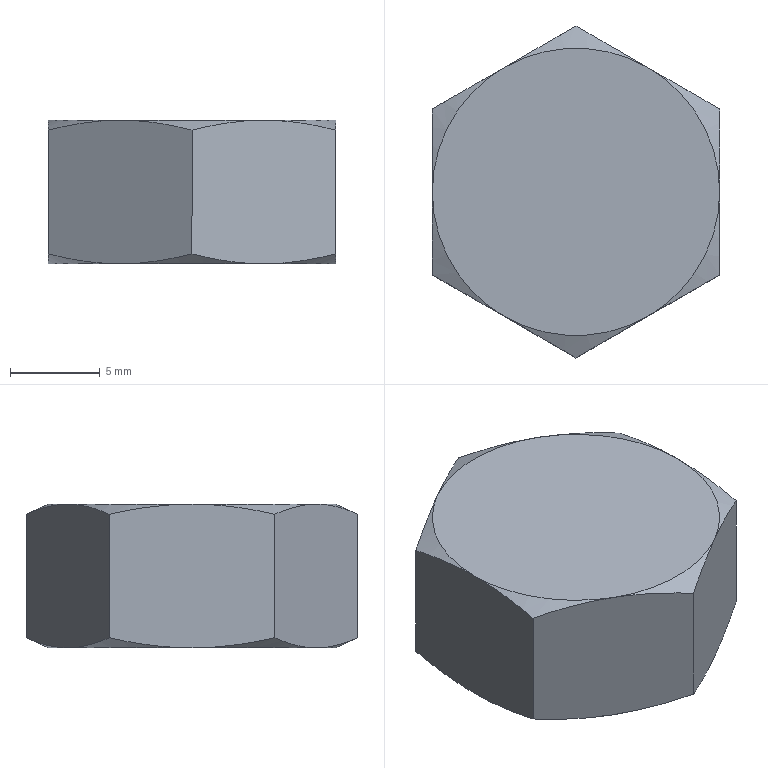Part | NX | features BREP 1 | 1 solid | 20 faces | box 16 x 18.475 x 8 mm | volume 1767 mm3 | cone 12 | plane 8
STEP:
#1=CARTESIAN_POINT('',(0.,-9.238,39.56));
#2=VERTEX_POINT('',#1);
#3=CARTESIAN_POINT('',(-4.,-6.928,39.));
#4=VERTEX_POINT('',#3);
#5=CARTESIAN_POINT('',(0.,-9.238,39.56));
#6=CARTESIAN_POINT('',(-1.317,-8.477,39.216));
#7=CARTESIAN_POINT('',(-2.647,-7.709,39.));
#8=CARTESIAN_POINT('',(-4.,-6.928,39.));
#9=B_SPLINE_CURVE_WITH_KNOTS('',3,(#5,#6,#7,#8),.UNSPECIFIED.,.F.,.F.,(4,4),(0.,0.004653),.UNSPECIFIED.);
#10=EDGE_CURVE('',#2,#4,#9,.T.);
#11=ORIENTED_EDGE('',*,*,#10,.T.);
#12=CARTESIAN_POINT('',(4.,-6.928,39.));
#13=VERTEX_POINT('',#12);
#14=CARTESIAN_POINT('',(0.,0.,39.));
#15=DIRECTION('',(0.,0.,-1.));
#16=DIRECTION('',(0.5,-0.866,0.));
#17=AXIS2_PLACEMENT_3D('',#14,#15,#16);
#18=CIRCLE('',#17,8.);
#19=EDGE_CURVE('',#13,#4,#18,.T.);
#20=ORIENTED_EDGE('',*,*,#19,.F.);
#21=CARTESIAN_POINT('',(4.,-6.928,39.));
#22=CARTESIAN_POINT('',(2.647,-7.709,39.));
#23=CARTESIAN_POINT('',(1.317,-8.477,39.216));
#24=CARTESIAN_POINT('',(0.,-9.238,39.56));
#25=B_SPLINE_CURVE_WITH_KNOTS('',3,(#21,#22,#23,#24),.UNSPECIFIED.,.F.,.F.,(4,4),(0.,0.004653),.UNSPECIFIED.);
#26=EDGE_CURVE('',#13,#2,#25,.T.);
#27=ORIENTED_EDGE('',*,*,#26,.T.);
#28=EDGE_LOOP('',(#11,#20,#27));
#29=FACE_BOUND('',#28,.T.);
#30=CARTESIAN_POINT('',(0.,0.,39.28));
#31=DIRECTION('',(0.,0.,1.));
#32=DIRECTION('',(-1.,0.,0.));
#33=AXIS2_PLACEMENT_3D('',#30,#31,#32);
#34=CONICAL_SURFACE('',#33,8.619,1.146);
#35=ADVANCED_FACE('',(#29),#34,.T.);
#36=CARTESIAN_POINT('',(0.,-9.238,46.44));
#37=VERTEX_POINT('',#36);
#38=CARTESIAN_POINT('',(0.,-9.238,39.56));
#39=DIRECTION('',(0.,0.,1.));
#40=VECTOR('',#39,1000.);
#41=LINE('',#38,#40);
#42=EDGE_CURVE('',#2,#37,#41,.T.);
#43=ORIENTED_EDGE('',*,*,#42,.F.);
#44=ORIENTED_EDGE('',*,*,#26,.F.);
#45=CARTESIAN_POINT('',(8.,-4.619,39.56));
#46=VERTEX_POINT('',#45);
#47=CARTESIAN_POINT('',(8.,-4.619,39.56));
#48=CARTESIAN_POINT('',(6.683,-5.379,39.216));
#49=CARTESIAN_POINT('',(5.353,-6.147,39.));
#50=CARTESIAN_POINT('',(4.,-6.928,39.));
#51=B_SPLINE_CURVE_WITH_KNOTS('',3,(#47,#48,#49,#50),.UNSPECIFIED.,.F.,.F.,(4,4),(0.,0.004653),.UNSPECIFIED.);
#52=EDGE_CURVE('',#46,#13,#51,.T.);
#53=ORIENTED_EDGE('',*,*,#52,.F.);
#54=CARTESIAN_POINT('',(8.,-4.619,46.44));
#55=VERTEX_POINT('',#54);
#56=CARTESIAN_POINT('',(8.,-4.619,39.56));
#57=DIRECTION('',(0.,0.,1.));
#58=VECTOR('',#57,1000.);
#59=LINE('',#56,#58);
#60=EDGE_CURVE('',#46,#55,#59,.T.);
#61=ORIENTED_EDGE('',*,*,#60,.T.);
#62=CARTESIAN_POINT('',(4.,-6.928,47.));
#63=VERTEX_POINT('',#62);
#64=CARTESIAN_POINT('',(4.,-6.928,47.));
#65=CARTESIAN_POINT('',(5.353,-6.147,47.));
#66=CARTESIAN_POINT('',(6.683,-5.379,46.784));
#67=CARTESIAN_POINT('',(8.,-4.619,46.44));
#68=B_SPLINE_CURVE_WITH_KNOTS('',3,(#64,#65,#66,#67),.UNSPECIFIED.,.F.,.F.,(4,4),(0.,0.004653),.UNSPECIFIED.);
#69=EDGE_CURVE('',#63,#55,#68,.T.);
#70=ORIENTED_EDGE('',*,*,#69,.F.);
#71=CARTESIAN_POINT('',(0.,-9.238,46.44));
#72=CARTESIAN_POINT('',(1.317,-8.477,46.784));
#73=CARTESIAN_POINT('',(2.647,-7.709,47.));
#74=CARTESIAN_POINT('',(4.,-6.928,47.));
#75=B_SPLINE_CURVE_WITH_KNOTS('',3,(#71,#72,#73,#74),.UNSPECIFIED.,.F.,.F.,(4,4),(0.,0.004653),.UNSPECIFIED.);
#76=EDGE_CURVE('',#37,#63,#75,.T.);
#77=ORIENTED_EDGE('',*,*,#76,.F.);
#78=EDGE_LOOP('',(#43,#44,#53,#61,#70,#77));
#79=FACE_BOUND('',#78,.T.);
#80=CARTESIAN_POINT('',(0.,-9.238,47.));
#81=DIRECTION('',(-0.5,0.866,0.));
#82=DIRECTION('',(0.866,0.5,0.));
#83=AXIS2_PLACEMENT_3D('',#80,#81,#82);
#84=PLANE('',#83);
#85=ADVANCED_FACE('',(#79),#84,.F.);
#86=ORIENTED_EDGE('',*,*,#76,.T.);
#87=CARTESIAN_POINT('',(-4.,-6.928,47.));
#88=VERTEX_POINT('',#87);
#89=CARTESIAN_POINT('',(0.,0.,47.));
#90=DIRECTION('',(0.,0.,1.));
#91=DIRECTION('',(-0.5,-0.866,0.));
#92=AXIS2_PLACEMENT_3D('',#89,#90,#91);
#93=CIRCLE('',#92,8.);
#94=EDGE_CURVE('',#88,#63,#93,.T.);
#95=ORIENTED_EDGE('',*,*,#94,.F.);
#96=CARTESIAN_POINT('',(-4.,-6.928,47.));
#97=CARTESIAN_POINT('',(-2.647,-7.709,47.));
#98=CARTESIAN_POINT('',(-1.317,-8.477,46.784));
#99=CARTESIAN_POINT('',(0.,-9.238,46.44));
#100=B_SPLINE_CURVE_WITH_KNOTS('',3,(#96,#97,#98,#99),.UNSPECIFIED.,.F.,.F.,(4,4),(0.,0.004653),.UNSPECIFIED.);
#101=EDGE_CURVE('',#88,#37,#100,.T.);
#102=ORIENTED_EDGE('',*,*,#101,.T.);
#103=EDGE_LOOP('',(#86,#95,#102));
#104=FACE_BOUND('',#103,.T.);
#105=CARTESIAN_POINT('',(0.,0.,46.72));
#106=DIRECTION('',(0.,0.,-1.));
#107=DIRECTION('',(1.,0.,0.));
#108=AXIS2_PLACEMENT_3D('',#105,#106,#107);
#109=CONICAL_SURFACE('',#108,8.619,1.146);
#110=ADVANCED_FACE('',(#104),#109,.T.);
#111=CARTESIAN_POINT('',(-8.,-4.619,39.56));
#112=VERTEX_POINT('',#111);
#113=CARTESIAN_POINT('',(-8.,-4.619,46.44));
#114=VERTEX_POINT('',#113);
#115=CARTESIAN_POINT('',(-8.,-4.619,39.56));
#116=DIRECTION('',(0.,0.,1.));
#117=VECTOR('',#116,1000.);
#118=LINE('',#115,#117);
#119=EDGE_CURVE('',#112,#114,#118,.T.);
#120=ORIENTED_EDGE('',*,*,#119,.F.);
#121=CARTESIAN_POINT('',(-4.,-6.928,39.));
#122=CARTESIAN_POINT('',(-5.353,-6.147,39.));
#123=CARTESIAN_POINT('',(-6.683,-5.379,39.216));
#124=CARTESIAN_POINT('',(-8.,-4.619,39.56));
#125=B_SPLINE_CURVE_WITH_KNOTS('',3,(#121,#122,#123,#124),.UNSPECIFIED.,.F.,.F.,(4,4),(0.,0.004653),.UNSPECIFIED.);
#126=EDGE_CURVE('',#4,#112,#125,.T.);
#127=ORIENTED_EDGE('',*,*,#126,.F.);
#128=ORIENTED_EDGE('',*,*,#10,.F.);
#129=ORIENTED_EDGE('',*,*,#42,.T.);
#130=ORIENTED_EDGE('',*,*,#101,.F.);
#131=CARTESIAN_POINT('',(-8.,-4.619,46.44));
#132=CARTESIAN_POINT('',(-6.683,-5.379,46.784));
#133=CARTESIAN_POINT('',(-5.353,-6.147,47.));
#134=CARTESIAN_POINT('',(-4.,-6.928,47.));
#135=B_SPLINE_CURVE_WITH_KNOTS('',3,(#131,#132,#133,#134),.UNSPECIFIED.,.F.,.F.,(4,4),(0.,0.004653),.UNSPECIFIED.);
#136=EDGE_CURVE('',#114,#88,#135,.T.);
#137=ORIENTED_EDGE('',*,*,#136,.F.);
#138=EDGE_LOOP('',(#120,#127,#128,#129,#130,#137));
#139=FACE_BOUND('',#138,.T.);
#140=CARTESIAN_POINT('',(-8.,-4.619,47.));
#141=DIRECTION('',(0.5,0.866,0.));
#142=DIRECTION('',(0.866,-0.5,0.));
#143=AXIS2_PLACEMENT_3D('',#140,#141,#142);
#144=PLANE('',#143);
#145=ADVANCED_FACE('',(#139),#144,.F.);
#146=CARTESIAN_POINT('',(-8.,0.,47.));
#147=VERTEX_POINT('',#146);
#148=CARTESIAN_POINT('',(0.,0.,47.));
#149=DIRECTION('',(0.,0.,1.));
#150=DIRECTION('',(-1.,0.,0.));
#151=AXIS2_PLACEMENT_3D('',#148,#149,#150);
#152=CIRCLE('',#151,8.);
#153=EDGE_CURVE('',#147,#88,#152,.T.);
#154=ORIENTED_EDGE('',*,*,#153,.F.);
#155=CARTESIAN_POINT('',(-8.,0.,47.));
#156=CARTESIAN_POINT('',(-8.,-1.562,47.));
#157=CARTESIAN_POINT('',(-8.,-3.098,46.784));
#158=CARTESIAN_POINT('',(-8.,-4.619,46.44));
#159=B_SPLINE_CURVE_WITH_KNOTS('',3,(#155,#156,#157,#158),.UNSPECIFIED.,.F.,.F.,(4,4),(0.,0.004653),.UNSPECIFIED.);
#160=EDGE_CURVE('',#147,#114,#159,.T.);
#161=ORIENTED_EDGE('',*,*,#160,.T.);
#162=ORIENTED_EDGE('',*,*,#136,.T.);
#163=EDGE_LOOP('',(#154,#161,#162));
#164=FACE_BOUND('',#163,.T.);
#165=CARTESIAN_POINT('',(0.,0.,46.72));
#166=DIRECTION('',(0.,0.,-1.));
#167=DIRECTION('',(1.,0.,0.));
#168=AXIS2_PLACEMENT_3D('',#165,#166,#167);
#169=CONICAL_SURFACE('',#168,8.619,1.146);
#170=ADVANCED_FACE('',(#164),#169,.T.);
#171=CARTESIAN_POINT('',(-8.,4.619,39.56));
#172=VERTEX_POINT('',#171);
#173=CARTESIAN_POINT('',(-8.,4.619,46.44));
#174=VERTEX_POINT('',#173);
#175=CARTESIAN_POINT('',(-8.,4.619,39.56));
#176=DIRECTION('',(0.,0.,1.));
#177=VECTOR('',#176,1000.);
#178=LINE('',#175,#177);
#179=EDGE_CURVE('',#172,#174,#178,.T.);
#180=ORIENTED_EDGE('',*,*,#179,.F.);
#181=CARTESIAN_POINT('',(-8.,0.,39.));
#182=VERTEX_POINT('',#181);
#183=CARTESIAN_POINT('',(-8.,0.,39.));
#184=CARTESIAN_POINT('',(-8.,1.562,39.));
#185=CARTESIAN_POINT('',(-8.,3.098,39.216));
#186=CARTESIAN_POINT('',(-8.,4.619,39.56));
#187=B_SPLINE_CURVE_WITH_KNOTS('',3,(#183,#184,#185,#186),.UNSPECIFIED.,.F.,.F.,(4,4),(0.,0.004653),.UNSPECIFIED.);
#188=EDGE_CURVE('',#182,#172,#187,.T.);
#189=ORIENTED_EDGE('',*,*,#188,.F.);
#190=CARTESIAN_POINT('',(-8.,-4.619,39.56));
#191=CARTESIAN_POINT('',(-8.,-3.098,39.216));
#192=CARTESIAN_POINT('',(-8.,-1.562,39.));
#193=CARTESIAN_POINT('',(-8.,0.,39.));
#194=B_SPLINE_CURVE_WITH_KNOTS('',3,(#190,#191,#192,#193),.UNSPECIFIED.,.F.,.F.,(4,4),(0.,0.004653),.UNSPECIFIED.);
#195=EDGE_CURVE('',#112,#182,#194,.T.);
#196=ORIENTED_EDGE('',*,*,#195,.F.);
#197=ORIENTED_EDGE('',*,*,#119,.T.);
#198=ORIENTED_EDGE('',*,*,#160,.F.);
#199=CARTESIAN_POINT('',(-8.,4.619,46.44));
#200=CARTESIAN_POINT('',(-8.,3.098,46.784));
#201=CARTESIAN_POINT('',(-8.,1.562,47.));
#202=CARTESIAN_POINT('',(-8.,0.,47.));
#203=B_SPLINE_CURVE_WITH_KNOTS('',3,(#199,#200,#201,#202),.UNSPECIFIED.,.F.,.F.,(4,4),(0.,0.004653),.UNSPECIFIED.);
#204=EDGE_CURVE('',#174,#147,#203,.T.);
#205=ORIENTED_EDGE('',*,*,#204,.F.);
#206=EDGE_LOOP('',(#180,#189,#196,#197,#198,#205));
#207=FACE_BOUND('',#206,.T.);
#208=CARTESIAN_POINT('',(-8.,4.619,47.));
#209=DIRECTION('',(1.,0.,0.));
#210=DIRECTION('',(0.,-1.,0.));
#211=AXIS2_PLACEMENT_3D('',#208,#209,#210);
#212=PLANE('',#211);
#213=ADVANCED_FACE('',(#207),#212,.F.);
#214=ORIENTED_EDGE('',*,*,#204,.T.);
#215=CARTESIAN_POINT('',(-4.,6.928,47.));
#216=VERTEX_POINT('',#215);
#217=CARTESIAN_POINT('',(0.,0.,47.));
#218=DIRECTION('',(0.,0.,1.));
#219=DIRECTION('',(-0.5,0.866,0.));
#220=AXIS2_PLACEMENT_3D('',#217,#218,#219);
#221=CIRCLE('',#220,8.);
#222=EDGE_CURVE('',#216,#147,#221,.T.);
#223=ORIENTED_EDGE('',*,*,#222,.F.);
#224=CARTESIAN_POINT('',(-4.,6.928,47.));
#225=CARTESIAN_POINT('',(-5.353,6.147,47.));
#226=CARTESIAN_POINT('',(-6.683,5.379,46.784));
#227=CARTESIAN_POINT('',(-8.,4.619,46.44));
#228=B_SPLINE_CURVE_WITH_KNOTS('',3,(#224,#225,#226,#227),.UNSPECIFIED.,.F.,.F.,(4,4),(0.,0.004653),.UNSPECIFIED.);
#229=EDGE_CURVE('',#216,#174,#228,.T.);
#230=ORIENTED_EDGE('',*,*,#229,.T.);
#231=EDGE_LOOP('',(#214,#223,#230));
#232=FACE_BOUND('',#231,.T.);
#233=CARTESIAN_POINT('',(0.,0.,46.72));
#234=DIRECTION('',(0.,0.,-1.));
#235=DIRECTION('',(1.,0.,0.));
#236=AXIS2_PLACEMENT_3D('',#233,#234,#235);
#237=CONICAL_SURFACE('',#236,8.619,1.146);
#238=ADVANCED_FACE('',(#232),#237,.T.);
#239=CARTESIAN_POINT('',(0.,9.238,39.56));
#240=VERTEX_POINT('',#239);
#241=CARTESIAN_POINT('',(0.,9.238,46.44));
#242=VERTEX_POINT('',#241);
#243=CARTESIAN_POINT('',(0.,9.238,39.56));
#244=DIRECTION('',(0.,0.,1.));
#245=VECTOR('',#244,1000.);
#246=LINE('',#243,#245);
#247=EDGE_CURVE('',#240,#242,#246,.T.);
#248=ORIENTED_EDGE('',*,*,#247,.F.);
#249=CARTESIAN_POINT('',(-4.,6.928,39.));
#250=VERTEX_POINT('',#249);
#251=CARTESIAN_POINT('',(-4.,6.928,39.));
#252=CARTESIAN_POINT('',(-2.647,7.709,39.));
#253=CARTESIAN_POINT('',(-1.317,8.477,39.216));
#254=CARTESIAN_POINT('',(0.,9.238,39.56));
#255=B_SPLINE_CURVE_WITH_KNOTS('',3,(#251,#252,#253,#254),.UNSPECIFIED.,.F.,.F.,(4,4),(0.,0.004653),.UNSPECIFIED.);
#256=EDGE_CURVE('',#250,#240,#255,.T.);
#257=ORIENTED_EDGE('',*,*,#256,.F.);
#258=CARTESIAN_POINT('',(-8.,4.619,39.56));
#259=CARTESIAN_POINT('',(-6.683,5.379,39.216));
#260=CARTESIAN_POINT('',(-5.353,6.147,39.));
#261=CARTESIAN_POINT('',(-4.,6.928,39.));
#262=B_SPLINE_CURVE_WITH_KNOTS('',3,(#258,#259,#260,#261),.UNSPECIFIED.,.F.,.F.,(4,4),(0.,0.004653),.UNSPECIFIED.);
#263=EDGE_CURVE('',#172,#250,#262,.T.);
#264=ORIENTED_EDGE('',*,*,#263,.F.);
#265=ORIENTED_EDGE('',*,*,#179,.T.);
#266=ORIENTED_EDGE('',*,*,#229,.F.);
#267=CARTESIAN_POINT('',(0.,9.238,46.44));
#268=CARTESIAN_POINT('',(-1.317,8.477,46.784));
#269=CARTESIAN_POINT('',(-2.647,7.709,47.));
#270=CARTESIAN_POINT('',(-4.,6.928,47.));
#271=B_SPLINE_CURVE_WITH_KNOTS('',3,(#267,#268,#269,#270),.UNSPECIFIED.,.F.,.F.,(4,4),(0.,0.004653),.UNSPECIFIED.);
#272=EDGE_CURVE('',#242,#216,#271,.T.);
#273=ORIENTED_EDGE('',*,*,#272,.F.);
#274=EDGE_LOOP('',(#248,#257,#264,#265,#266,#273));
#275=FACE_BOUND('',#274,.T.);
#276=CARTESIAN_POINT('',(0.,9.238,47.));
#277=DIRECTION('',(0.5,-0.866,0.));
#278=DIRECTION('',(-0.866,-0.5,0.));
#279=AXIS2_PLACEMENT_3D('',#276,#277,#278);
#280=PLANE('',#279);
#281=ADVANCED_FACE('',(#275),#280,.F.);
#282=ORIENTED_EDGE('',*,*,#272,.T.);
#283=CARTESIAN_POINT('',(4.,6.928,47.));
#284=VERTEX_POINT('',#283);
#285=CARTESIAN_POINT('',(0.,0.,47.));
#286=DIRECTION('',(0.,0.,1.));
#287=DIRECTION('',(0.5,0.866,0.));
#288=AXIS2_PLACEMENT_3D('',#285,#286,#287);
#289=CIRCLE('',#288,8.);
#290=EDGE_CURVE('',#284,#216,#289,.T.);
#291=ORIENTED_EDGE('',*,*,#290,.F.);
#292=CARTESIAN_POINT('',(4.,6.928,47.));
#293=CARTESIAN_POINT('',(2.647,7.709,47.));
#294=CARTESIAN_POINT('',(1.317,8.477,46.784));
#295=CARTESIAN_POINT('',(0.,9.238,46.44));
#296=B_SPLINE_CURVE_WITH_KNOTS('',3,(#292,#293,#294,#295),.UNSPECIFIED.,.F.,.F.,(4,4),(0.,0.004653),.UNSPECIFIED.);
#297=EDGE_CURVE('',#284,#242,#296,.T.);
#298=ORIENTED_EDGE('',*,*,#297,.T.);
#299=EDGE_LOOP('',(#282,#291,#298));
#300=FACE_BOUND('',#299,.T.);
#301=CARTESIAN_POINT('',(0.,0.,46.72));
#302=DIRECTION('',(0.,0.,-1.));
#303=DIRECTION('',(1.,0.,0.));
#304=AXIS2_PLACEMENT_3D('',#301,#302,#303);
#305=CONICAL_SURFACE('',#304,8.619,1.146);
#306=ADVANCED_FACE('',(#300),#305,.T.);
#307=CARTESIAN_POINT('',(8.,4.619,39.56));
#308=VERTEX_POINT('',#307);
#309=CARTESIAN_POINT('',(8.,4.619,46.44));
#310=VERTEX_POINT('',#309);
#311=CARTESIAN_POINT('',(8.,4.619,39.56));
#312=DIRECTION('',(0.,0.,1.));
#313=VECTOR('',#312,1000.);
#314=LINE('',#311,#313);
#315=EDGE_CURVE('',#308,#310,#314,.T.);
#316=ORIENTED_EDGE('',*,*,#315,.F.);
#317=CARTESIAN_POINT('',(4.,6.928,39.));
#318=VERTEX_POINT('',#317);
#319=CARTESIAN_POINT('',(4.,6.928,39.));
#320=CARTESIAN_POINT('',(5.353,6.147,39.));
#321=CARTESIAN_POINT('',(6.683,5.379,39.216));
#322=CARTESIAN_POINT('',(8.,4.619,39.56));
#323=B_SPLINE_CURVE_WITH_KNOTS('',3,(#319,#320,#321,#322),.UNSPECIFIED.,.F.,.F.,(4,4),(0.,0.004653),.UNSPECIFIED.);
#324=EDGE_CURVE('',#318,#308,#323,.T.);
#325=ORIENTED_EDGE('',*,*,#324,.F.);
#326=CARTESIAN_POINT('',(0.,9.238,39.56));
#327=CARTESIAN_POINT('',(1.317,8.477,39.216));
#328=CARTESIAN_POINT('',(2.647,7.709,39.));
#329=CARTESIAN_POINT('',(4.,6.928,39.));
#330=B_SPLINE_CURVE_WITH_KNOTS('',3,(#326,#327,#328,#329),.UNSPECIFIED.,.F.,.F.,(4,4),(0.,0.004653),.UNSPECIFIED.);
#331=EDGE_CURVE('',#240,#318,#330,.T.);
#332=ORIENTED_EDGE('',*,*,#331,.F.);
#333=ORIENTED_EDGE('',*,*,#247,.T.);
#334=ORIENTED_EDGE('',*,*,#297,.F.);
#335=CARTESIAN_POINT('',(8.,4.619,46.44));
#336=CARTESIAN_POINT('',(6.683,5.379,46.784));
#337=CARTESIAN_POINT('',(5.353,6.147,47.));
#338=CARTESIAN_POINT('',(4.,6.928,47.));
#339=B_SPLINE_CURVE_WITH_KNOTS('',3,(#335,#336,#337,#338),.UNSPECIFIED.,.F.,.F.,(4,4),(0.,0.004653),.UNSPECIFIED.);
#340=EDGE_CURVE('',#310,#284,#339,.T.);
#341=ORIENTED_EDGE('',*,*,#340,.F.);
#342=EDGE_LOOP('',(#316,#325,#332,#333,#334,#341));
#343=FACE_BOUND('',#342,.T.);
#344=CARTESIAN_POINT('',(8.,4.619,47.));
#345=DIRECTION('',(-0.5,-0.866,0.));
#346=DIRECTION('',(-0.866,0.5,0.));
#347=AXIS2_PLACEMENT_3D('',#344,#345,#346);
#348=PLANE('',#347);
#349=ADVANCED_FACE('',(#343),#348,.F.);
#350=ORIENTED_EDGE('',*,*,#340,.T.);
#351=CARTESIAN_POINT('',(8.,0.,47.));
#352=VERTEX_POINT('',#351);
#353=CARTESIAN_POINT('',(0.,0.,47.));
#354=DIRECTION('',(0.,0.,1.));
#355=DIRECTION('',(1.,0.,0.));
#356=AXIS2_PLACEMENT_3D('',#353,#354,#355);
#357=CIRCLE('',#356,8.);
#358=EDGE_CURVE('',#352,#284,#357,.T.);
#359=ORIENTED_EDGE('',*,*,#358,.F.);
#360=CARTESIAN_POINT('',(8.,0.,47.));
#361=CARTESIAN_POINT('',(8.,1.562,47.));
#362=CARTESIAN_POINT('',(8.,3.098,46.784));
#363=CARTESIAN_POINT('',(8.,4.619,46.44));
#364=B_SPLINE_CURVE_WITH_KNOTS('',3,(#360,#361,#362,#363),.UNSPECIFIED.,.F.,.F.,(4,4),(0.,0.004653),.UNSPECIFIED.);
#365=EDGE_CURVE('',#352,#310,#364,.T.);
#366=ORIENTED_EDGE('',*,*,#365,.T.);
#367=EDGE_LOOP('',(#350,#359,#366));
#368=FACE_BOUND('',#367,.T.);
#369=CARTESIAN_POINT('',(0.,0.,46.72));
#370=DIRECTION('',(0.,0.,-1.));
#371=DIRECTION('',(1.,0.,0.));
#372=AXIS2_PLACEMENT_3D('',#369,#370,#371);
#373=CONICAL_SURFACE('',#372,8.619,1.146);
#374=ADVANCED_FACE('',(#368),#373,.T.);
#375=ORIENTED_EDGE('',*,*,#60,.F.);
#376=CARTESIAN_POINT('',(8.,0.,39.));
#377=VERTEX_POINT('',#376);
#378=CARTESIAN_POINT('',(8.,0.,39.));
#379=CARTESIAN_POINT('',(8.,-1.562,39.));
#380=CARTESIAN_POINT('',(8.,-3.098,39.216));
#381=CARTESIAN_POINT('',(8.,-4.619,39.56));
#382=B_SPLINE_CURVE_WITH_KNOTS('',3,(#378,#379,#380,#381),.UNSPECIFIED.,.F.,.F.,(4,4),(0.,0.004653),.UNSPECIFIED.);
#383=EDGE_CURVE('',#377,#46,#382,.T.);
#384=ORIENTED_EDGE('',*,*,#383,.F.);
#385=CARTESIAN_POINT('',(8.,4.619,39.56));
#386=CARTESIAN_POINT('',(8.,3.098,39.216));
#387=CARTESIAN_POINT('',(8.,1.562,39.));
#388=CARTESIAN_POINT('',(8.,0.,39.));
#389=B_SPLINE_CURVE_WITH_KNOTS('',3,(#385,#386,#387,#388),.UNSPECIFIED.,.F.,.F.,(4,4),(0.,0.004653),.UNSPECIFIED.);
#390=EDGE_CURVE('',#308,#377,#389,.T.);
#391=ORIENTED_EDGE('',*,*,#390,.F.);
#392=ORIENTED_EDGE('',*,*,#315,.T.);
#393=ORIENTED_EDGE('',*,*,#365,.F.);
#394=CARTESIAN_POINT('',(8.,-4.619,46.44));
#395=CARTESIAN_POINT('',(8.,-3.098,46.784));
#396=CARTESIAN_POINT('',(8.,-1.562,47.));
#397=CARTESIAN_POINT('',(8.,0.,47.));
#398=B_SPLINE_CURVE_WITH_KNOTS('',3,(#394,#395,#396,#397),.UNSPECIFIED.,.F.,.F.,(4,4),(0.,0.004653),.UNSPECIFIED.);
#399=EDGE_CURVE('',#55,#352,#398,.T.);
#400=ORIENTED_EDGE('',*,*,#399,.F.);
#401=EDGE_LOOP('',(#375,#384,#391,#392,#393,#400));
#402=FACE_BOUND('',#401,.T.);
#403=CARTESIAN_POINT('',(8.,-4.619,47.));
#404=DIRECTION('',(-1.,0.,0.));
#405=DIRECTION('',(0.,0.,-1.));
#406=AXIS2_PLACEMENT_3D('',#403,#404,#405);
#407=PLANE('',#406);
#408=ADVANCED_FACE('',(#402),#407,.F.);
#409=ORIENTED_EDGE('',*,*,#399,.T.);
#410=CARTESIAN_POINT('',(0.,0.,47.));
#411=DIRECTION('',(0.,0.,1.));
#412=DIRECTION('',(0.5,-0.866,0.));
#413=AXIS2_PLACEMENT_3D('',#410,#411,#412);
#414=CIRCLE('',#413,8.);
#415=EDGE_CURVE('',#63,#352,#414,.T.);
#416=ORIENTED_EDGE('',*,*,#415,.F.);
#417=ORIENTED_EDGE('',*,*,#69,.T.);
#418=EDGE_LOOP('',(#409,#416,#417));
#419=FACE_BOUND('',#418,.T.);
#420=CARTESIAN_POINT('',(0.,0.,46.72));
#421=DIRECTION('',(0.,0.,-1.));
#422=DIRECTION('',(1.,0.,0.));
#423=AXIS2_PLACEMENT_3D('',#420,#421,#422);
#424=CONICAL_SURFACE('',#423,8.619,1.146);
#425=ADVANCED_FACE('',(#419),#424,.T.);
#426=ORIENTED_EDGE('',*,*,#358,.T.);
#427=ORIENTED_EDGE('',*,*,#290,.T.);
#428=ORIENTED_EDGE('',*,*,#222,.T.);
#429=ORIENTED_EDGE('',*,*,#153,.T.);
#430=ORIENTED_EDGE('',*,*,#94,.T.);
#431=ORIENTED_EDGE('',*,*,#415,.T.);
#432=EDGE_LOOP('',(#426,#427,#428,#429,#430,#431));
#433=FACE_BOUND('',#432,.T.);
#434=CARTESIAN_POINT('',(0.,0.,47.));
#435=DIRECTION('',(0.,0.,1.));
#436=DIRECTION('',(-1.,0.,0.));
#437=AXIS2_PLACEMENT_3D('',#434,#435,#436);
#438=PLANE('',#437);
#439=ADVANCED_FACE('',(#433),#438,.T.);
#440=CARTESIAN_POINT('',(0.,0.,39.));
#441=DIRECTION('',(0.,0.,-1.));
#442=DIRECTION('',(0.5,0.866,0.));
#443=AXIS2_PLACEMENT_3D('',#440,#441,#442);
#444=CIRCLE('',#443,8.);
#445=EDGE_CURVE('',#318,#377,#444,.T.);
#446=ORIENTED_EDGE('',*,*,#445,.F.);
#447=ORIENTED_EDGE('',*,*,#324,.T.);
#448=ORIENTED_EDGE('',*,*,#390,.T.);
#449=EDGE_LOOP('',(#446,#447,#448));
#450=FACE_BOUND('',#449,.T.);
#451=CARTESIAN_POINT('',(0.,0.,39.28));
#452=DIRECTION('',(0.,0.,1.));
#453=DIRECTION('',(-1.,0.,0.));
#454=AXIS2_PLACEMENT_3D('',#451,#452,#453);
#455=CONICAL_SURFACE('',#454,8.619,1.146);
#456=ADVANCED_FACE('',(#450),#455,.T.);
#457=CARTESIAN_POINT('',(0.,0.,39.));
#458=DIRECTION('',(0.,0.,-1.));
#459=DIRECTION('',(1.,0.,0.));
#460=AXIS2_PLACEMENT_3D('',#457,#458,#459);
#461=CIRCLE('',#460,8.);
#462=EDGE_CURVE('',#377,#13,#461,.T.);
#463=ORIENTED_EDGE('',*,*,#462,.T.);
#464=ORIENTED_EDGE('',*,*,#19,.T.);
#465=CARTESIAN_POINT('',(0.,0.,39.));
#466=DIRECTION('',(0.,0.,-1.));
#467=DIRECTION('',(-0.5,-0.866,0.));
#468=AXIS2_PLACEMENT_3D('',#465,#466,#467);
#469=CIRCLE('',#468,8.);
#470=EDGE_CURVE('',#4,#182,#469,.T.);
#471=ORIENTED_EDGE('',*,*,#470,.T.);
#472=CARTESIAN_POINT('',(0.,0.,39.));
#473=DIRECTION('',(0.,0.,-1.));
#474=DIRECTION('',(-1.,0.,0.));
#475=AXIS2_PLACEMENT_3D('',#472,#473,#474);
#476=CIRCLE('',#475,8.);
#477=EDGE_CURVE('',#182,#250,#476,.T.);
#478=ORIENTED_EDGE('',*,*,#477,.T.);
#479=CARTESIAN_POINT('',(0.,0.,39.));
#480=DIRECTION('',(0.,0.,-1.));
#481=DIRECTION('',(-0.5,0.866,0.));
#482=AXIS2_PLACEMENT_3D('',#479,#480,#481);
#483=CIRCLE('',#482,8.);
#484=EDGE_CURVE('',#250,#318,#483,.T.);
#485=ORIENTED_EDGE('',*,*,#484,.T.);
#486=ORIENTED_EDGE('',*,*,#445,.T.);
#487=EDGE_LOOP('',(#463,#464,#471,#478,#485,#486));
#488=FACE_BOUND('',#487,.T.);
#489=CARTESIAN_POINT('',(0.,0.,39.));
#490=DIRECTION('',(0.,0.,1.));
#491=DIRECTION('',(-1.,0.,0.));
#492=AXIS2_PLACEMENT_3D('',#489,#490,#491);
#493=PLANE('',#492);
#494=ADVANCED_FACE('',(#488),#493,.F.);
#495=ORIENTED_EDGE('',*,*,#484,.F.);
#496=ORIENTED_EDGE('',*,*,#256,.T.);
#497=ORIENTED_EDGE('',*,*,#331,.T.);
#498=EDGE_LOOP('',(#495,#496,#497));
#499=FACE_BOUND('',#498,.T.);
#500=CARTESIAN_POINT('',(0.,0.,39.28));
#501=DIRECTION('',(0.,0.,1.));
#502=DIRECTION('',(-1.,0.,0.));
#503=AXIS2_PLACEMENT_3D('',#500,#501,#502);
#504=CONICAL_SURFACE('',#503,8.619,1.146);
#505=ADVANCED_FACE('',(#499),#504,.T.);
#506=ORIENTED_EDGE('',*,*,#477,.F.);
#507=ORIENTED_EDGE('',*,*,#188,.T.);
#508=ORIENTED_EDGE('',*,*,#263,.T.);
#509=EDGE_LOOP('',(#506,#507,#508));
#510=FACE_BOUND('',#509,.T.);
#511=CARTESIAN_POINT('',(0.,0.,39.28));
#512=DIRECTION('',(0.,0.,1.));
#513=DIRECTION('',(-1.,0.,0.));
#514=AXIS2_PLACEMENT_3D('',#511,#512,#513);
#515=CONICAL_SURFACE('',#514,8.619,1.146);
#516=ADVANCED_FACE('',(#510),#515,.T.);
#517=ORIENTED_EDGE('',*,*,#195,.T.);
#518=ORIENTED_EDGE('',*,*,#470,.F.);
#519=ORIENTED_EDGE('',*,*,#126,.T.);
#520=EDGE_LOOP('',(#517,#518,#519));
#521=FACE_BOUND('',#520,.T.);
#522=CARTESIAN_POINT('',(0.,0.,39.28));
#523=DIRECTION('',(0.,0.,1.));
#524=DIRECTION('',(-1.,0.,0.));
#525=AXIS2_PLACEMENT_3D('',#522,#523,#524);
#526=CONICAL_SURFACE('',#525,8.619,1.146);
#527=ADVANCED_FACE('',(#521),#526,.T.);
#528=ORIENTED_EDGE('',*,*,#52,.T.);
#529=ORIENTED_EDGE('',*,*,#462,.F.);
#530=ORIENTED_EDGE('',*,*,#383,.T.);
#531=EDGE_LOOP('',(#528,#529,#530));
#532=FACE_BOUND('',#531,.T.);
#533=CARTESIAN_POINT('',(0.,0.,39.28));
#534=DIRECTION('',(0.,0.,1.));
#535=DIRECTION('',(-1.,0.,0.));
#536=AXIS2_PLACEMENT_3D('',#533,#534,#535);
#537=CONICAL_SURFACE('',#536,8.619,1.146);
#538=ADVANCED_FACE('',(#532),#537,.T.);
#539=CLOSED_SHELL('',(#35,#85,#110,#145,#170,#213,#238,#281,#306,#349,#374,#408,#425,#439,#456,#494,#505,#516,#527,#538));
#540=MANIFOLD_SOLID_BREP('',#539);
#541=(LENGTH_UNIT()NAMED_UNIT(*)SI_UNIT(.MILLI.,.METRE.));
#542=UNCERTAINTY_MEASURE_WITH_UNIT(LENGTH_MEASURE(0.0508),#541,'','');
#543=(NAMED_UNIT(*)PLANE_ANGLE_UNIT()SI_UNIT($,.RADIAN.));
#544=(NAMED_UNIT(*)SI_UNIT($,.STERADIAN.)SOLID_ANGLE_UNIT());
#545=(GEOMETRIC_REPRESENTATION_CONTEXT(3)GLOBAL_UNCERTAINTY_ASSIGNED_CONTEXT((#542))GLOBAL_UNIT_ASSIGNED_CONTEXT((#541,#543,#544))REPRESENTATION_CONTEXT('',''));
#546=ADVANCED_BREP_SHAPE_REPRESENTATION('',(#540),#545);